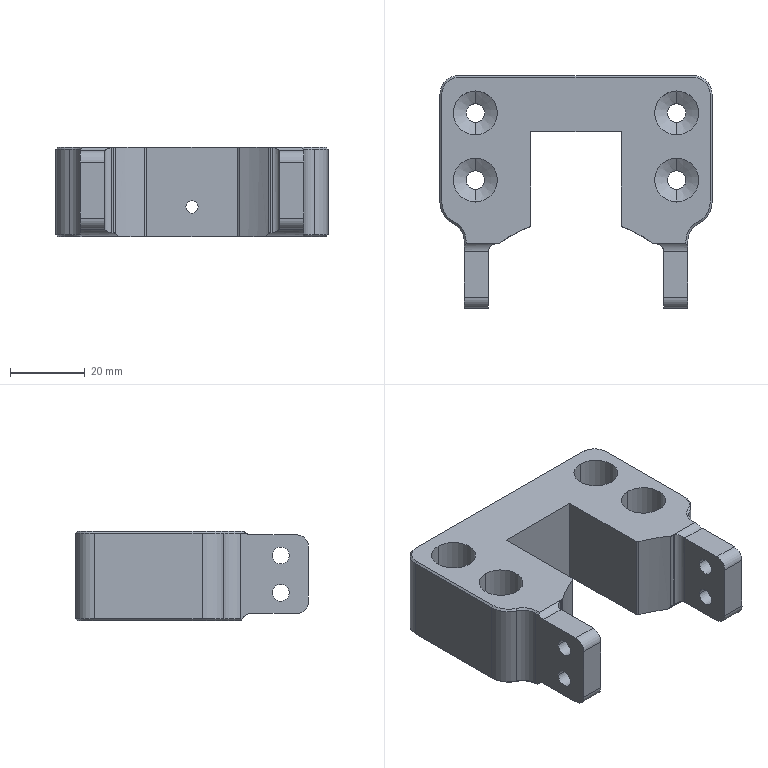NC program | NX | posted with a generic post | part box 73 x 62.4 x 24 mm
Lines 5233 to 5455 of 11507:
(ZLEVEL_PROFILE_COPY_COPY_1 , TOOL : D10JING)
N10410 T11 M6
N10412 G54
N10414 G17 G0 G90 X-33.154 Y37.075 S8000 M3
N10416 G43 Z30. H11
N10418 Z-11.
N10420 G94 G1 Z-12. F800.
N10422 G3 X-31.5 Y36.2 R2.
N10424 G1 X31.5
N10426 G2 X41.5 Y26.2 R10.
N10428 G1 Y-2.7
N10430 G2 X35. Y-13.056 R11.5
N10432 G1 Y-31.193
N10434 G2 X30. Y-36.2 R5.
N10436 G1 X23.5
N10438 G2 X18.5 Y-31.2 R5.
N10440 G1 Y-18.309
N10442 G2 X17.614 Y-17.78 R6.
N10444 G3 X10.842 Y-14.117 R30.15
N10446 G2 X7.6 Y-11.134 R6.
N10448 X7.1 Y-8.954 R5.
N10450 G1 Y11.2
N10452 X-7.1
N10454 Y-8.954
N10456 G2 X-7.6 Y-11.134 R5.
N10458 X-10.842 Y-14.117 R6.
N10460 G3 X-17.614 Y-17.78 R30.15
N10462 G2 X-18.501 Y-18.309 R6.
N10464 G1 X-18.5 Y-18.357
N10466 Y-31.2
N10468 G2 X-23.5 Y-36.2 R5.
N10470 G1 X-30.
N10472 G2 X-35. Y-31.2 R5.
N10474 G1 Y-13.056
N10476 G2 X-41.5 Y-2.7 R11.5
N10478 G1 Y26.2
N10480 G2 X-31.5 Y36.2 R10.
N10482 G3 X-29.768 Y37.2 R2.
N10484 G1 Z-11.
N10486 G0 X-33.154 Y37.075 Z-23.
N10488 G1 Z-24.
N10490 G3 X-31.5 Y36.2 R2.
N10492 G1 X31.5
N10494 G2 X41.5 Y26.2 R10.
N10496 G1 Y-2.7
N10498 G2 X35. Y-13.056 R11.5
N10500 G1 Y-31.193
N10502 G2 X30. Y-36.2 R5.
N10504 G1 X23.5
N10506 G2 X18.5 Y-31.2 R5.
N10508 G1 Y-18.309
N10510 G2 X17.614 Y-17.78 R6.
N10512 G3 X10.842 Y-14.117 R30.15
N10514 G2 X7.6 Y-11.134 R6.
N10516 X7.1 Y-8.954 R5.
N10518 G1 Y11.2
N10520 X-7.1
N10522 Y-8.954
N10524 G2 X-7.6 Y-11.134 R5.
N10526 X-10.842 Y-14.117 R6.
N10528 G3 X-17.614 Y-17.78 R30.15
N10530 G2 X-18.5 Y-18.309 R6.
N10532 G1 Y-18.358
N10534 Y-31.2
N10536 G2 X-23.5 Y-36.2 R5.
N10538 G1 X-30.
N10540 G2 X-35. Y-31.2 R5.
N10542 G1 Y-13.066
N10544 Y-13.056
N10546 G2 X-41.5 Y-2.7 R11.5
N10548 G1 Y26.2
N10550 G2 X-31.5 Y36.2 R10.
N10552 G3 X-29.768 Y37.2 R2.
N10554 G1 Z-23.
N10556 G0 Z30.
(FLOOR_WALL_1_1_COPY , TOOL : D10JING)
N10558 X-17.36 Y-34.175 S7000
N10560 Z0.5
N10562 G1 Z-1. F1250.
N10564 X-17.634 Y-33.7
N10566 G3 X-18.5 Y-33.2 R1.
N10568 G1 X-35.
N10570 Y-29.152
N10572 X-18.5
N10574 Y-25.104
N10576 X-35.
N10578 Y-21.056
N10580 X-18.5
N10582 G2 X-17.634 Y-21.556 R1.
N10584 G1 X-17. Y-22.654
N10586 Z0.5
N10588 G0 Z30.
N10590 X36.14 Y-34.175
N10592 Z0.5
N10594 G1 Z-1.
N10596 X35.866 Y-33.7
N10598 G3 X35. Y-33.2 R1.
N10600 G1 X18.5
N10602 Y-29.152
N10604 X35.
N10606 Y-25.104
N10608 X18.5
N10610 Y-21.056
N10612 X35.
N10614 G2 X35.866 Y-21.556 R1.
N10616 G1 X36.5 Y-22.654
N10618 Z0.5
N10620 G0 Z30.
(ZLEVEL_PROFILE_COPY_COPY_1_COPY , TOOL : D10JING)
N10622 G55
N10624 X-33.154 Y37.075 S8000
N10626 Z-11.
N10628 G1 Z-12. F800.
N10630 G3 X-31.5 Y36.2 R2.
N10632 G1 X31.5
N10634 G2 X41.5 Y26.2 R10.
N10636 G1 Y-2.7
N10638 G2 X35. Y-13.056 R11.5
N10640 G1 Y-31.193
N10642 G2 X30. Y-36.2 R5.
N10644 G1 X23.5
N10646 G2 X18.5 Y-31.2 R5.
N10648 G1 Y-18.309
N10650 G2 X17.614 Y-17.78 R6.
N10652 G3 X10.842 Y-14.117 R30.15
N10654 G2 X7.6 Y-11.134 R6.
N10656 X7.1 Y-8.954 R5.
N10658 G1 Y11.2
N10660 X-7.1
N10662 Y-8.954
N10664 G2 X-7.6 Y-11.134 R5.
N10666 X-10.842 Y-14.117 R6.
N10668 G3 X-17.614 Y-17.78 R30.15
N10670 G2 X-18.501 Y-18.309 R6.
N10672 G1 X-18.5 Y-18.357
N10674 Y-31.2
N10676 G2 X-23.5 Y-36.2 R5.
N10678 G1 X-30.
N10680 G2 X-35. Y-31.2 R5.
N10682 G1 Y-13.056
N10684 G2 X-41.5 Y-2.7 R11.5
N10686 G1 Y26.2
N10688 G2 X-31.5 Y36.2 R10.
N10690 G3 X-29.768 Y37.2 R2.
N10692 G1 Z-11.
N10694 G0 X-33.154 Y37.075 Z-23.
N10696 G1 Z-24.
N10698 G3 X-31.5 Y36.2 R2.
N10700 G1 X31.5
N10702 G2 X41.5 Y26.2 R10.
N10704 G1 Y-2.7
N10706 G2 X35. Y-13.056 R11.5
N10708 G1 Y-31.193
N10710 G2 X30. Y-36.2 R5.
N10712 G1 X23.5
N10714 G2 X18.5 Y-31.2 R5.
N10716 G1 Y-18.309
N10718 G2 X17.614 Y-17.78 R6.
N10720 G3 X10.842 Y-14.117 R30.15
N10722 G2 X7.6 Y-11.134 R6.
N10724 X7.1 Y-8.954 R5.
N10726 G1 Y11.2
N10728 X-7.1
N10730 Y-8.954
N10732 G2 X-7.6 Y-11.134 R5.
N10734 X-10.842 Y-14.117 R6.
N10736 G3 X-17.614 Y-17.78 R30.15
N10738 G2 X-18.5 Y-18.309 R6.
N10740 G1 Y-18.358
N10742 Y-31.2
N10744 G2 X-23.5 Y-36.2 R5.
N10746 G1 X-30.
N10748 G2 X-35. Y-31.2 R5.
N10750 G1 Y-13.066
N10752 Y-13.056
N10754 G2 X-41.5 Y-2.7 R11.5
N10756 G1 Y26.2
N10758 G2 X-31.5 Y36.2 R10.
N10760 G3 X-29.768 Y37.2 R2.
N10762 G1 Z-23.
N10764 G0 Z30.
(FLOOR_WALL_1_1_COPY_COPY_1 , TOOL : D10JING)
N10766 X-17.36 Y-34.175 S7000
N10768 Z0.5
N10770 G1 Z-1. F1250.
N10772 X-17.634 Y-33.7
N10774 G3 X-18.5 Y-33.2 R1.
N10776 G1 X-35.
N10778 Y-29.152
N10780 X-18.5
N10782 Y-25.104
N10784 X-35.
N10786 Y-21.056
N10788 X-18.5
N10790 G2 X-17.634 Y-21.556 R1.
N10792 G1 X-17. Y-22.654
N10794 Z0.5
N10796 G0 Z30.
N10798 X36.14 Y-34.175
N10800 Z0.5
N10802 G1 Z-1.
N10804 X35.866 Y-33.7
N10806 G3 X35. Y-33.2 R1.
N10808 G1 X18.5
N10810 Y-29.152
N10812 X35.
N10814 Y-25.104
N10816 X18.5
N10818 Y-21.056
N10820 X35.
N10822 G2 X35.866 Y-21.556 R1.
N10824 G1 X36.5 Y-22.654
N10826 Z0.5
N10828 G0 Z30.
N10830 M5